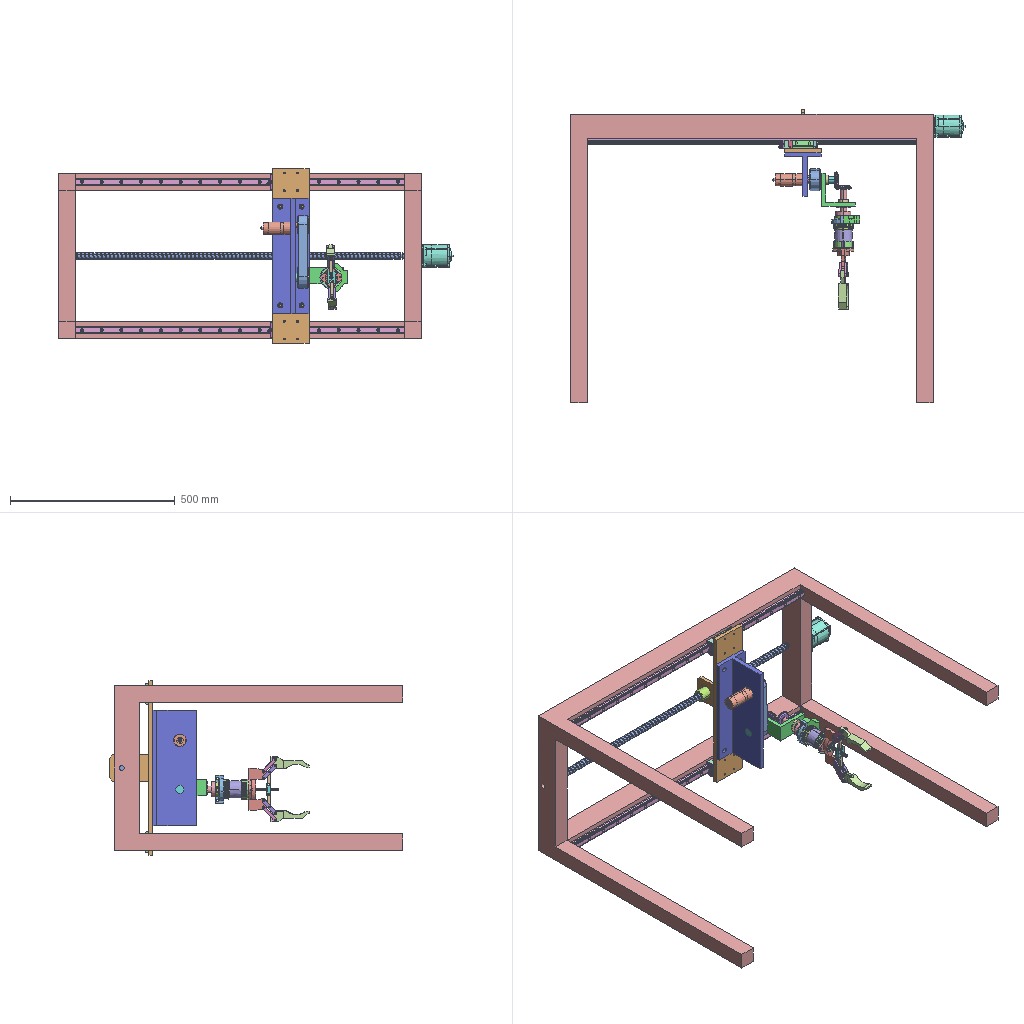Assembly | SolidWorks | 38 different items | 51 placed | box 1198 x 890 x 530 mm
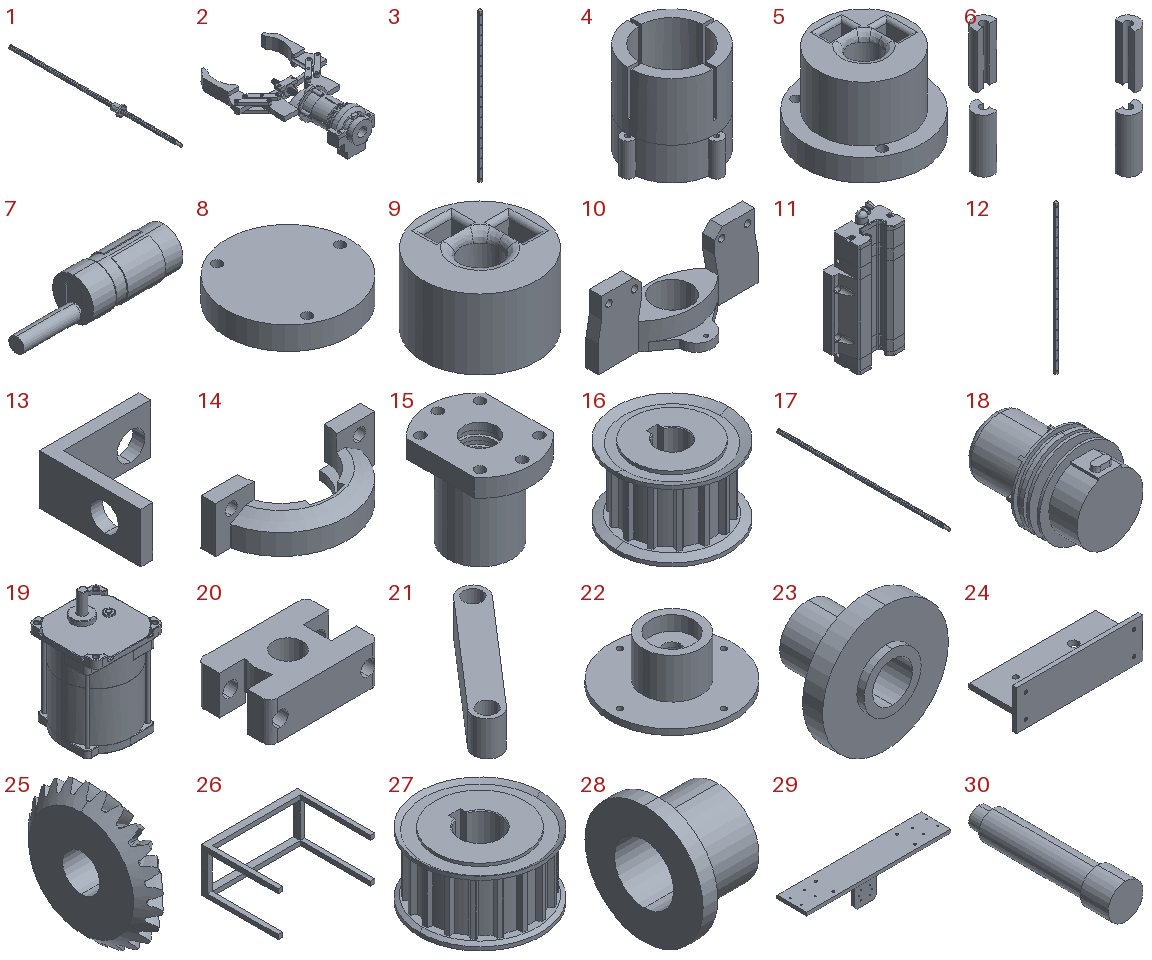Parts list (item | name | quantity | parent item | size | volume | features):
1 | (subassembly) | x1 | - | 58 x 1028 x 57.544 mm | 346833 mm3 | features AEMSimFeature 1
2 | (subassembly) | x1 | - | 197.047 x 296.861 x 84.62 mm | 451687 mm3 | features CompositeCurve 13, ReferencePattern 8, MirrorCompFeat 3, RefAxis 2
3 | (subassembly) | x2 | - | 20 x 17.5 x 1000 mm | 300247 mm3 | -
4 | (subassembly) | x1 | in 2 | 61.8 x 61.8 x 55 mm | 44978 mm3 | -
5 | (subassembly) | x1 | in 2 | 32 x 32 x 21 mm | 10117 mm3 | -
6 | - | x1 | in 4 | 61.8 x 61.8 x 20 mm | 2131 mm3 | features BaseBody 4
7 | - | x1 | - | 144.5 x 38 x 38 mm | 99346 mm3 | features ICE 13, Fillet 4, Cut 2, Split 2, Chamfer 1, CreateAssemFeat 1, Extrusion 1, MirrorPattern 1, Revolution 1
8 | - | x1 | in 5 | 32 x 32 x 6 mm | 4734 mm3 | features BaseBody 1
9 | - | x1 | in 5 | 24.4 x 24.4 x 15 mm | 5383 mm3 | features BaseBody 1
10 | - | x1 | in 2 | 127 x 64 x 52.75 mm | 56573 mm3 | features ICE 6, Chamfer 1, Cut 1, Extrusion 1, MirrorPattern 1
11 | - | x2 | - | 63 x 25.7 x 118.4 mm | 108820 mm3 | features ICE 22, Extrusion 5, MirrorPattern 5, Fillet 4, MirrorSolid 4, Chamfer 3, RevCut 3, Dome 2, LPattern 2, Revolution 2, DeleteBody 1, LibraryFeature 1
12 | - | x2 | in 3 | 20 x 17.5 x 1000 mm | 300247 mm3 | features ICE 19, MirrorPattern 5, Extrusion 4, MirrorSolid 4, Chamfer 3, Fillet 3, RevCut 3, Dome 2, LPattern 2, DeleteBody 1, LibraryFeature 1, Revolution 1
13 | - | x1 | - | 100 x 102 x 50 mm | 99222 mm3 | features ICE 3, Extrusion 1, MoveFace 1
14 | - | x1 | in 2 | 84.091 x 34.963 x 24.206 mm | 18007 mm3 | features ICE 14, 3DProfileFeature 1, Cut 1, Extrusion 1, Fillet 1, HoleWzd 1, MirrorPattern 1, MirrorSolid 1, RefAxis 1, RevCut 1, Revolution 1, SewRefSurface 1, Sweep 1, Thicken 1
15 | - | x1 | in 1 | 44 x 58 x 51 mm | 47513 mm3 | features Extrusion 1, Helix 1, ICE 1, RefAxis 1, SweepCut 1
16 | - | x1 | - | 52 x 52 x 32.5 mm | 36076 mm3 | features ICE 10, Chamfer 9, RevCut 3, CirPattern 2, Revolution 2
17 | - | x1 | in 1 | 20 x 1028 x 20 mm | 299367 mm3 | features Revolution 2, Helix 1, MoveFace 1, SweepCut 1
18 | - | x1 | in 2 | 58.42 x 91.643 x 58.42 mm | 118735 mm3 | features ICE 14, Fillet 2, CirPattern 1, Cut 1, Extrusion 1, RefAxis 1, RevCut 1
19 | - | x1 | - | 67.25 x 67.25 x 118.75 mm | 309581 mm3 | features ICE 20, Fillet 6, Extrusion 1, RevCut 1
20 | - | x1 | in 2 | 38.1 x 25.4 x 13.5 mm | 7968 mm3 | features Cut 2, ICE 2, Extrusion 1, Fillet 1
21 | - | x2 | in 2 | 32.522 x 36.456 x 9.652 mm | 2831 mm3 | features Extrusion 1
22 | - | x1 | in 2 | 64 x 64 x 24 mm | 13940 mm3 | features Fillet 1, HoleWzd 1, ICE 1, RevCut 1, Revolution 1
23 | - | x1 | in 2 | 22 x 14.75 x 22 mm | 1646 mm3 | features ICE 2, 3DProfileFeature 1, Extrusion 1, HoleWzd 1
24 | - | x1 | - | 350 x 132 x 110 mm | 1033847 mm3 | features Cut 2, Extrusion 1, HoleWzd 1, ICE 1
25 | - | x2 | - | 12.427 x 50.574 x 50.574 mm | 13201 mm3 | features 3DProfileFeature 12, BlendCut 1, CirPattern 1, ICE 1, RefAxis 1, Revolution 1
26 | - | x1 | - | 1100 x 875 x 500 mm | 19232329 mm3 | features Cut 1, Extrusion 1, ICE 1
27 | - | x1 | - | 61 x 61 x 32.5 mm | 59006 mm3 | features ICE 10, Chamfer 9, RevCut 3, CirPattern 2, Revolution 2
28 | - | x2 | - | 25 x 40 x 40 mm | 10744 mm3 | features Revolution 1
29 | - | x1 | - | 530 x 110 x 132 mm | 790668 mm3 | features HoleWzd 2, Chamfer 1, Cut 1, Extrusion 1, ICE 1
30 | - | x1 | - | 25 x 105 x 25 mm | 34919 mm3 | features ICE 2, Extrusion 1
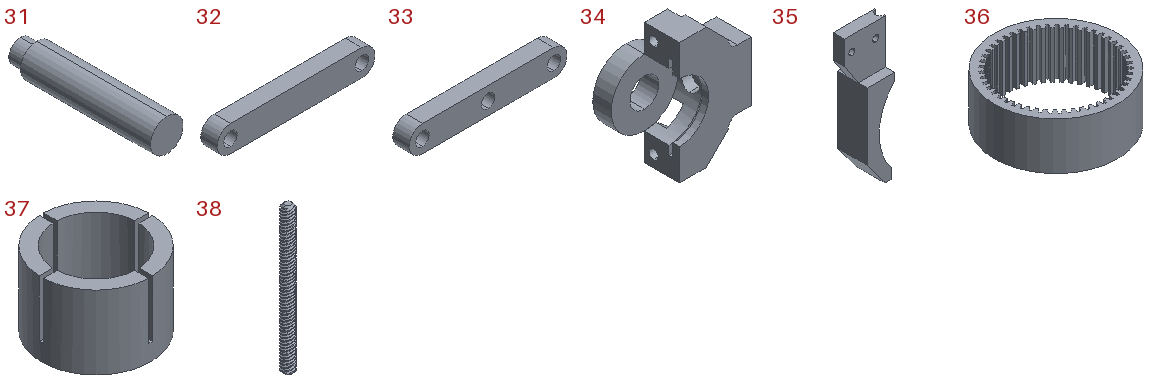31 | - | x1 | - | 20 x 90 x 20 mm | 26672 mm3 | features ICE 4, Extrusion 1, MirrorPattern 1
32 | - | x4 | in 2 | 60.96 x 6.35 x 10.16 mm | 3522 mm3 | features Extrusion 1, ICE 1
33 | - | x4 | in 2 | 60.96 x 6.35 x 10.16 mm | 3387 mm3 | features ICE 2, Extrusion 1
34 | - | x1 | in 2 | 72.644 x 36.906 x 84.074 mm | 68724 mm3 | features ICE 19, MirrorPattern 3, 3DProfileFeature 2, Fillet 2, RefAxis 2, Chamfer 1, CombineBodies 1, Cut 1, Extrusion 1, HoleWzd 1, MirrorSolid 1, MoveCopyBody 1, Stock 1
35 | - | x2 | in 2 | 35.052 x 25.4 x 115.945 mm | 36905 mm3 | features ICE 2, Extrusion 1
36 | - | x1 | in 4 | 52 x 52 x 20 mm | 11731 mm3 | features BaseBody 1
37 | - | x1 | in 4 | 52 x 52 x 35 mm | 31115 mm3 | features BaseBody 1, Cut 1
38 | - | x1 | in 2 | 8 x 8 x 101.6 mm | 3914 mm3 | features Helix 4, Sweep 4, RevCut 2, Extrusion 1, ICE 1
Mates (type | each side: item.copy, entity, surface, feature):
In the top assembly
Concentric | 26.1 face cylinder Cut-Extrude1 | 17.1 face cylinder Revolve2
Coincident | 26.1 face plane Boss-Extrude1 | 17.1 edge
Coincident | 26.1 face plane Boss-Extrude1 | 12.1 face plane Boss-Extrude10
Width | 12.1 face plane Boss-Extrude10 | 12.1 face plane Boss-Extrude10 | 26.1 face plane Boss-Extrude1 | 26.1 face plane Boss-Extrude1
Coincident | 26.1 face plane Boss-Extrude2 | 12.1 face plane Boss-Extrude10
Coincident | 26.1 face plane Boss-Extrude1 | 12.2 face plane Boss-Extrude10
Coincident | 26.1 face plane Boss-Extrude2 | 12.2 face plane Boss-Extrude10
Width | 12.2 face plane Boss-Extrude10 | 12.2 face plane Boss-Extrude10 | 26.1 face plane Boss-Extrude1 | 26.1 face plane Boss-Extrude1
Concentric | 26.1 face cylinder Cut-Extrude1 | 19.1 face cylinder Boss-Extrude14
Coincident | 26.1 face plane Boss-Extrude1 | 19.1 face plane Boss-Extrude12
Parallel | 26.1 face plane Boss-Extrude1 | 19.1 face plane Boss-Extrude10
Coincident | 15.1 face plane Boss-Extrude1 | 29.1 face plane Boss-Extrude1
Parallel | 15.1 face plane Boss-Extrude1 | 29.1 face plane Boss-Extrude1
Width | 29.1 face plane Boss-Extrude2 | 29.1 face plane Boss-Extrude2 | 26.1 face plane Boss-Extrude1 | 26.1 face plane Boss-Extrude1
DistanceDim | 26.1 face plane Boss-Extrude1 | 29.1 face plane Boss-Extrude2
Concentric | 29.1 face cylinder M5 Tapped Hole1 | 11.1 face cylinder Mirror1
Concentric | 29.1 face cylinder M5 Tapped Hole1 | 11.1 face cylinder Cut-Revolve1
Coincident | 29.1 face plane Boss-Extrude2 | 11.1 face plane Boss-Extrude1
Concentric | 29.1 face cylinder M5 Tapped Hole1 | 11.2 face cylinder Mirror1
Coincident | 29.1 face plane Boss-Extrude2 | 11.2 face plane Boss-Extrude1
Concentric | 29.1 face cylinder M5 Tapped Hole1 | 11.2 face cylinder Cut-Revolve1
Coincident | 29.1 face plane Boss-Extrude2 | 24.1 face plane Boss-Extrude1 | 2 times
Width | 24.1 face plane Boss-Extrude1 | 24.1 face plane Boss-Extrude1 | 29.1 face plane Boss-Extrude2 | 29.1 face plane Boss-Extrude2
Concentric | 7.1 face cylinder Boss-Extrude10 | 24.1 face cylinder Cut-Extrude1
Coincident | 7.1 face plane Boss-Extrude2 | 24.1 face plane Boss-Extrude2
Concentric | 7.1 face cylinder Boss-Extrude10 | 16.1 face cylinder Cut-Extrude2
Coincident | 7.1 face plane Boss-Extrude10 | 16.1 face plane Revolve1
Concentric | 24.1 face cylinder Cut-Extrude2 | 27.1 face cylinder Cut-Extrude2
Concentric | 24.1 face cylinder Cut-Extrude2 | 30.1 face cylinder Boss-Extrude1
Coincident | 24.1 face plane Boss-Extrude2 | 30.1 face plane Boss-Extrude1
Coincident | 27.1 face plane Revolve1 | 30.1 face plane Boss-Extrude1
Concentric | 30.1 face cylinder Boss-Extrude2 | 28.1 face cylinder Revolve1
Coincident | 27.1 face plane Revolve1 | 28.1 face plane Revolve1
Concentric | 30.1 face cylinder Boss-Extrude3 | 25.1 face cylinder Cut-Extrude1
Coincident | 30.1 face plane Boss-Extrude3 | 25.1 face plane Revolve1
Coincident | 25.1 select_type:25 | 25.2 select_type:25
Concentric | 28.1 face cylinder Revolve1 | 13.1 face cylinder Cut-Extrude1
Parallel | 24.1 face plane Boss-Extrude1 | 13.1 face plane Boss-Extrude1
Coincident | 28.1 face plane Revolve1 | 13.1 face plane Boss-Extrude1
Parallel | 25.2 face plane Revolve1 | 13.1 face plane Boss-Extrude2
Concentric | 13.1 face cylinder Cut-Extrude2 | 28.2 face cylinder Revolve1
Coincident | 13.1 face plane Boss-Extrude1 | 28.2 face plane Revolve1
Concentric | 25.2 face cylinder Cut-Extrude1 | 31.1 face cylinder Boss-Extrude3
Coincident | 25.2 face plane Revolve1 | 31.1 face plane Boss-Extrude2
BeltDim | 16.1 edge | 27.1 edge
Concentric | 31.1 face cylinder Boss-Extrude1 | 18.1 face cylinder Boss-Extrude1
Coincident | 31.1 face plane Boss-Extrude1 | 34.1 edge
In subassembly 1
Concentric | 17.2 face cylinder Revolve1 | 15.2 face cylinder Boss-Extrude2
Screw | 17.2 face cylinder Revolve1 | 15.2 face cylinder Boss-Extrude1
In subassembly 2
Concentric | 18.2 face cylinder Boss-Extrude7 | 9.1 face cylinder Imported1
Concentric | 18.2 face cylinder Boss-Extrude3 | 37.1 face cylinder Imported1
Coincident | 18.2 face plane Boss-Extrude3 | 36.1 face plane Imported1
Concentric | 9.1 face cylinder Imported1 | 22.1 face cylinder Cut-Revolve1
Coincident | 36.1 face plane Imported1 | 22.1 face plane Revolve1
Concentric | 6.1 face cylinder Imported1 | 22.1 face cylinder Ø2.8 (2.8) Diameter Hole1
InPlace | 22.1 face plane Boss-Extrude1 | 10.1 plane
Coincident | 18.2 face plane Boss-Extrude3 | 8.1 face plane Imported1
Parallel | 18.2 face plane Boss-Extrude9 | 10.1 face plane Cut-Extrude6
Concentric | 9.1 edge | 38.1 edge
Coincident | 18.2 face plane Boss-Extrude7 | 38.1 face plane Boss-Extrude1
Concentric | 23.1 face cylinder M8x1.0 Tapped Hole1 | 38.1 edge
Coincident | 10.1 face plane Cut-Extrude6 | 35.1 face plane Boss-Extrude2
Parallel | 10.1 face plane Boss-Extrude1 | 35.1 face plane Boss-Extrude1
Concentric | 32.1 edge | 10.1 edge
Coincident | 10.1 face plane Cut-Extrude6 | 32.1 face plane Boss-Extrude1
Concentric | 35.1 edge | 32.1 edge
InPlace | 23.1 face plane Boss-Extrude1 | 20.1 plane
Parallel | 18.2 face plane Boss-Extrude9 | 20.1 face plane Boss-Extrude1
Concentric | 10.1 edge | 33.1 edge
Coincident | 10.1 face plane Cut-Extrude6 | 33.1 face plane Boss-Extrude1
Concentric | 35.1 edge | 33.1 edge
Concentric | 20.1 edge | 21.1 edge
Coincident | 20.1 face plane Cut-Extrude2 | 21.1 face plane Boss-Extrude1
Concentric | 21.1 face cylinder Boss-Extrude1 | 33.1 face cylinder Cut-Extrude1
LimitDistanceDim | 20.1 face plane Boss-Extrude1 | 10.1 face plane Boss-Extrude1
LimitDistanceDim | 35.2 face plane Boss-Extrude1 | 35.1 face plane Boss-Extrude1
Concentric | 18.2 face cylinder Boss-Extrude1 | 34.2 face cylinder MotorClip_V2_right
Parallel | 18.2 face plane Boss-Extrude9 | 34.2 face plane MotorClip_V2_right
Coincident | 18.2 face plane Boss-Extrude10 | 34.2 face plane Cut-Extrude5
Coincident | 34.2 face plane MotorClip_V2_right | 14.1 face plane Cut-Extrude9
Concentric | 18.2 face cylinder Boss-Extrude1 | 14.1 face cylinder Boss-Extrude1
Coincident | 34.2 face plane MotorClip_V2_right | 14.1 face plane Boss-Extrude1